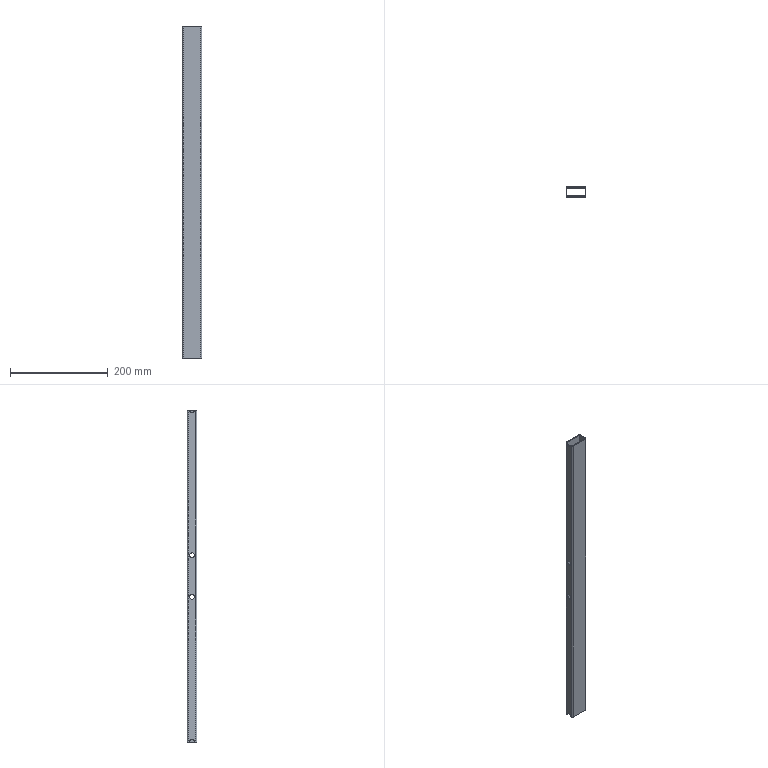Part | STEP file | 6150103 | 1 solid | 24 faces | box 40 x 20 x 680 mm | volume 112626 mm3 | cylinder 14 | plane 10 | commonest cylinder face diameters 10 x6 2 x4 5 x4
STEP:
#1=CARTESIAN_POINT('',(-18.5,-5.,340.));
#2=VERTEX_POINT('',#1);
#3=CARTESIAN_POINT('',(-18.5,-7.5,340.));
#4=VERTEX_POINT('',#3);
#5=CARTESIAN_POINT('',(-18.5,7.5,340.));
#6=DIRECTION('',(0.,-1.,0.));
#7=VECTOR('',#6,1000.);
#8=LINE('',#5,#7);
#9=EDGE_CURVE('',#2,#4,#8,.T.);
#10=ORIENTED_EDGE('',*,*,#9,.F.);
#11=CARTESIAN_POINT('',(-20.,-5.,340.));
#12=VERTEX_POINT('',#11);
#13=CARTESIAN_POINT('',(-10.,-5.,340.));
#14=DIRECTION('',(-1.,0.,0.));
#15=VECTOR('',#14,1000.);
#16=LINE('',#13,#15);
#17=EDGE_CURVE('',#2,#12,#16,.T.);
#18=ORIENTED_EDGE('',*,*,#17,.T.);
#19=CARTESIAN_POINT('',(-20.,-7.5,340.));
#20=VERTEX_POINT('',#19);
#21=CARTESIAN_POINT('',(-20.,7.5,340.));
#22=DIRECTION('',(0.,-1.,0.));
#23=VECTOR('',#22,1000.);
#24=LINE('',#21,#23);
#25=EDGE_CURVE('',#12,#20,#24,.T.);
#26=ORIENTED_EDGE('',*,*,#25,.T.);
#27=CARTESIAN_POINT('',(-17.5,-10.,340.));
#28=VERTEX_POINT('',#27);
#29=CARTESIAN_POINT('',(-17.5,-7.5,340.));
#30=DIRECTION('',(0.,0.,1.));
#31=DIRECTION('',(1.,0.,0.));
#32=AXIS2_PLACEMENT_3D('',#29,#30,#31);
#33=CIRCLE('',#32,2.5);
#34=EDGE_CURVE('',#20,#28,#33,.T.);
#35=ORIENTED_EDGE('',*,*,#34,.T.);
#36=CARTESIAN_POINT('',(17.5,-10.,340.));
#37=VERTEX_POINT('',#36);
#38=CARTESIAN_POINT('',(-17.5,-10.,340.));
#39=DIRECTION('',(1.,0.,0.));
#40=VECTOR('',#39,1000.);
#41=LINE('',#38,#40);
#42=EDGE_CURVE('',#28,#37,#41,.T.);
#43=ORIENTED_EDGE('',*,*,#42,.T.);
#44=CARTESIAN_POINT('',(20.,-7.5,340.));
#45=VERTEX_POINT('',#44);
#46=CARTESIAN_POINT('',(17.5,-7.5,340.));
#47=DIRECTION('',(0.,0.,1.));
#48=DIRECTION('',(1.,0.,0.));
#49=AXIS2_PLACEMENT_3D('',#46,#47,#48);
#50=CIRCLE('',#49,2.5);
#51=EDGE_CURVE('',#37,#45,#50,.T.);
#52=ORIENTED_EDGE('',*,*,#51,.T.);
#53=CARTESIAN_POINT('',(20.,7.5,340.));
#54=VERTEX_POINT('',#53);
#55=CARTESIAN_POINT('',(20.,7.5,340.));
#56=DIRECTION('',(0.,1.,0.));
#57=VECTOR('',#56,1000.);
#58=LINE('',#55,#57);
#59=EDGE_CURVE('',#45,#54,#58,.T.);
#60=ORIENTED_EDGE('',*,*,#59,.T.);
#61=CARTESIAN_POINT('',(17.5,10.,340.));
#62=VERTEX_POINT('',#61);
#63=CARTESIAN_POINT('',(17.5,7.5,340.));
#64=DIRECTION('',(0.,0.,1.));
#65=DIRECTION('',(-1.,0.,0.));
#66=AXIS2_PLACEMENT_3D('',#63,#64,#65);
#67=CIRCLE('',#66,2.5);
#68=EDGE_CURVE('',#54,#62,#67,.T.);
#69=ORIENTED_EDGE('',*,*,#68,.T.);
#70=CARTESIAN_POINT('',(-17.5,10.,340.));
#71=VERTEX_POINT('',#70);
#72=CARTESIAN_POINT('',(-17.5,10.,340.));
#73=DIRECTION('',(-1.,0.,0.));
#74=VECTOR('',#73,1000.);
#75=LINE('',#72,#74);
#76=EDGE_CURVE('',#62,#71,#75,.T.);
#77=ORIENTED_EDGE('',*,*,#76,.T.);
#78=CARTESIAN_POINT('',(-20.,7.5,340.));
#79=VERTEX_POINT('',#78);
#80=CARTESIAN_POINT('',(-17.5,7.5,340.));
#81=DIRECTION('',(0.,0.,1.));
#82=DIRECTION('',(1.,0.,0.));
#83=AXIS2_PLACEMENT_3D('',#80,#81,#82);
#84=CIRCLE('',#83,2.5);
#85=EDGE_CURVE('',#71,#79,#84,.T.);
#86=ORIENTED_EDGE('',*,*,#85,.T.);
#87=CARTESIAN_POINT('',(-20.,5.,340.));
#88=VERTEX_POINT('',#87);
#89=CARTESIAN_POINT('',(-20.,7.5,340.));
#90=DIRECTION('',(0.,-1.,0.));
#91=VECTOR('',#90,1000.);
#92=LINE('',#89,#91);
#93=EDGE_CURVE('',#79,#88,#92,.T.);
#94=ORIENTED_EDGE('',*,*,#93,.T.);
#95=CARTESIAN_POINT('',(-18.5,5.,340.));
#96=VERTEX_POINT('',#95);
#97=CARTESIAN_POINT('',(-10.,5.,340.));
#98=DIRECTION('',(1.,0.,0.));
#99=VECTOR('',#98,1000.);
#100=LINE('',#97,#99);
#101=EDGE_CURVE('',#88,#96,#100,.T.);
#102=ORIENTED_EDGE('',*,*,#101,.T.);
#103=CARTESIAN_POINT('',(-18.5,7.5,340.));
#104=VERTEX_POINT('',#103);
#105=CARTESIAN_POINT('',(-18.5,7.5,340.));
#106=DIRECTION('',(0.,-1.,0.));
#107=VECTOR('',#106,1000.);
#108=LINE('',#105,#107);
#109=EDGE_CURVE('',#104,#96,#108,.T.);
#110=ORIENTED_EDGE('',*,*,#109,.F.);
#111=CARTESIAN_POINT('',(-17.5,8.5,340.));
#112=VERTEX_POINT('',#111);
#113=CARTESIAN_POINT('',(-17.5,7.5,340.));
#114=DIRECTION('',(0.,0.,1.));
#115=DIRECTION('',(1.,0.,0.));
#116=AXIS2_PLACEMENT_3D('',#113,#114,#115);
#117=CIRCLE('',#116,1.);
#118=EDGE_CURVE('',#112,#104,#117,.T.);
#119=ORIENTED_EDGE('',*,*,#118,.F.);
#120=CARTESIAN_POINT('',(17.5,8.5,340.));
#121=VERTEX_POINT('',#120);
#122=CARTESIAN_POINT('',(-17.5,8.5,340.));
#123=DIRECTION('',(-1.,0.,0.));
#124=VECTOR('',#123,1000.);
#125=LINE('',#122,#124);
#126=EDGE_CURVE('',#121,#112,#125,.T.);
#127=ORIENTED_EDGE('',*,*,#126,.F.);
#128=CARTESIAN_POINT('',(18.5,7.5,340.));
#129=VERTEX_POINT('',#128);
#130=CARTESIAN_POINT('',(17.5,7.5,340.));
#131=DIRECTION('',(0.,0.,1.));
#132=DIRECTION('',(-1.,0.,0.));
#133=AXIS2_PLACEMENT_3D('',#130,#131,#132);
#134=CIRCLE('',#133,1.);
#135=EDGE_CURVE('',#129,#121,#134,.T.);
#136=ORIENTED_EDGE('',*,*,#135,.F.);
#137=CARTESIAN_POINT('',(18.5,-7.5,340.));
#138=VERTEX_POINT('',#137);
#139=CARTESIAN_POINT('',(18.5,7.5,340.));
#140=DIRECTION('',(0.,1.,0.));
#141=VECTOR('',#140,1000.);
#142=LINE('',#139,#141);
#143=EDGE_CURVE('',#138,#129,#142,.T.);
#144=ORIENTED_EDGE('',*,*,#143,.F.);
#145=CARTESIAN_POINT('',(17.5,-8.5,340.));
#146=VERTEX_POINT('',#145);
#147=CARTESIAN_POINT('',(17.5,-7.5,340.));
#148=DIRECTION('',(0.,0.,1.));
#149=DIRECTION('',(1.,0.,0.));
#150=AXIS2_PLACEMENT_3D('',#147,#148,#149);
#151=CIRCLE('',#150,1.);
#152=EDGE_CURVE('',#146,#138,#151,.T.);
#153=ORIENTED_EDGE('',*,*,#152,.F.);
#154=CARTESIAN_POINT('',(-17.5,-8.5,340.));
#155=VERTEX_POINT('',#154);
#156=CARTESIAN_POINT('',(-17.5,-8.5,340.));
#157=DIRECTION('',(1.,0.,0.));
#158=VECTOR('',#157,1000.);
#159=LINE('',#156,#158);
#160=EDGE_CURVE('',#155,#146,#159,.T.);
#161=ORIENTED_EDGE('',*,*,#160,.F.);
#162=CARTESIAN_POINT('',(-17.5,-7.5,340.));
#163=DIRECTION('',(0.,0.,1.));
#164=DIRECTION('',(1.,0.,0.));
#165=AXIS2_PLACEMENT_3D('',#162,#163,#164);
#166=CIRCLE('',#165,1.);
#167=EDGE_CURVE('',#4,#155,#166,.T.);
#168=ORIENTED_EDGE('',*,*,#167,.F.);
#169=EDGE_LOOP('',(#10,#18,#26,#35,#43,#52,#60,#69,#77,#86,#94,#102,#110,#119,#127,#136,#144,#153,#161,#168));
#170=FACE_OUTER_BOUND('',#169,.T.);
#171=CARTESIAN_POINT('',(17.5,7.5,340.));
#172=DIRECTION('',(0.,0.,-1.));
#173=DIRECTION('',(-1.,0.,0.));
#174=AXIS2_PLACEMENT_3D('',#171,#172,#173);
#175=PLANE('',#174);
#176=ADVANCED_FACE('',(#170),#175,.F.);
#177=CARTESIAN_POINT('',(-18.5,-5.,-340.));
#178=VERTEX_POINT('',#177);
#179=CARTESIAN_POINT('',(-20.,-5.,-340.));
#180=VERTEX_POINT('',#179);
#181=CARTESIAN_POINT('',(-10.,-5.,-340.));
#182=DIRECTION('',(-1.,0.,0.));
#183=VECTOR('',#182,1000.);
#184=LINE('',#181,#183);
#185=EDGE_CURVE('',#178,#180,#184,.T.);
#186=ORIENTED_EDGE('',*,*,#185,.F.);
#187=CARTESIAN_POINT('',(-18.5,-7.5,-340.));
#188=VERTEX_POINT('',#187);
#189=CARTESIAN_POINT('',(-18.5,7.5,-340.));
#190=DIRECTION('',(0.,-1.,0.));
#191=VECTOR('',#190,1000.);
#192=LINE('',#189,#191);
#193=EDGE_CURVE('',#178,#188,#192,.T.);
#194=ORIENTED_EDGE('',*,*,#193,.T.);
#195=CARTESIAN_POINT('',(-17.5,-8.5,-340.));
#196=VERTEX_POINT('',#195);
#197=CARTESIAN_POINT('',(-17.5,-7.5,-340.));
#198=DIRECTION('',(0.,0.,1.));
#199=DIRECTION('',(1.,0.,0.));
#200=AXIS2_PLACEMENT_3D('',#197,#198,#199);
#201=CIRCLE('',#200,1.);
#202=EDGE_CURVE('',#188,#196,#201,.T.);
#203=ORIENTED_EDGE('',*,*,#202,.T.);
#204=CARTESIAN_POINT('',(17.5,-8.5,-340.));
#205=VERTEX_POINT('',#204);
#206=CARTESIAN_POINT('',(-17.5,-8.5,-340.));
#207=DIRECTION('',(1.,0.,0.));
#208=VECTOR('',#207,1000.);
#209=LINE('',#206,#208);
#210=EDGE_CURVE('',#196,#205,#209,.T.);
#211=ORIENTED_EDGE('',*,*,#210,.T.);
#212=CARTESIAN_POINT('',(18.5,-7.5,-340.));
#213=VERTEX_POINT('',#212);
#214=CARTESIAN_POINT('',(17.5,-7.5,-340.));
#215=DIRECTION('',(0.,0.,1.));
#216=DIRECTION('',(1.,0.,0.));
#217=AXIS2_PLACEMENT_3D('',#214,#215,#216);
#218=CIRCLE('',#217,1.);
#219=EDGE_CURVE('',#205,#213,#218,.T.);
#220=ORIENTED_EDGE('',*,*,#219,.T.);
#221=CARTESIAN_POINT('',(18.5,7.5,-340.));
#222=VERTEX_POINT('',#221);
#223=CARTESIAN_POINT('',(18.5,7.5,-340.));
#224=DIRECTION('',(0.,1.,0.));
#225=VECTOR('',#224,1000.);
#226=LINE('',#223,#225);
#227=EDGE_CURVE('',#213,#222,#226,.T.);
#228=ORIENTED_EDGE('',*,*,#227,.T.);
#229=CARTESIAN_POINT('',(17.5,8.5,-340.));
#230=VERTEX_POINT('',#229);
#231=CARTESIAN_POINT('',(17.5,7.5,-340.));
#232=DIRECTION('',(0.,0.,1.));
#233=DIRECTION('',(-1.,0.,0.));
#234=AXIS2_PLACEMENT_3D('',#231,#232,#233);
#235=CIRCLE('',#234,1.);
#236=EDGE_CURVE('',#222,#230,#235,.T.);
#237=ORIENTED_EDGE('',*,*,#236,.T.);
#238=CARTESIAN_POINT('',(-17.5,8.5,-340.));
#239=VERTEX_POINT('',#238);
#240=CARTESIAN_POINT('',(-17.5,8.5,-340.));
#241=DIRECTION('',(-1.,0.,0.));
#242=VECTOR('',#241,1000.);
#243=LINE('',#240,#242);
#244=EDGE_CURVE('',#230,#239,#243,.T.);
#245=ORIENTED_EDGE('',*,*,#244,.T.);
#246=CARTESIAN_POINT('',(-18.5,7.5,-340.));
#247=VERTEX_POINT('',#246);
#248=CARTESIAN_POINT('',(-17.5,7.5,-340.));
#249=DIRECTION('',(0.,0.,1.));
#250=DIRECTION('',(1.,0.,0.));
#251=AXIS2_PLACEMENT_3D('',#248,#249,#250);
#252=CIRCLE('',#251,1.);
#253=EDGE_CURVE('',#239,#247,#252,.T.);
#254=ORIENTED_EDGE('',*,*,#253,.T.);
#255=CARTESIAN_POINT('',(-18.5,5.,-340.));
#256=VERTEX_POINT('',#255);
#257=CARTESIAN_POINT('',(-18.5,7.5,-340.));
#258=DIRECTION('',(0.,-1.,0.));
#259=VECTOR('',#258,1000.);
#260=LINE('',#257,#259);
#261=EDGE_CURVE('',#247,#256,#260,.T.);
#262=ORIENTED_EDGE('',*,*,#261,.T.);
#263=CARTESIAN_POINT('',(-20.,5.,-340.));
#264=VERTEX_POINT('',#263);
#265=CARTESIAN_POINT('',(-10.,5.,-340.));
#266=DIRECTION('',(1.,0.,0.));
#267=VECTOR('',#266,1000.);
#268=LINE('',#265,#267);
#269=EDGE_CURVE('',#264,#256,#268,.T.);
#270=ORIENTED_EDGE('',*,*,#269,.F.);
#271=CARTESIAN_POINT('',(-20.,7.5,-340.));
#272=VERTEX_POINT('',#271);
#273=CARTESIAN_POINT('',(-20.,7.5,-340.));
#274=DIRECTION('',(0.,-1.,0.));
#275=VECTOR('',#274,1000.);
#276=LINE('',#273,#275);
#277=EDGE_CURVE('',#272,#264,#276,.T.);
#278=ORIENTED_EDGE('',*,*,#277,.F.);
#279=CARTESIAN_POINT('',(-17.5,10.,-340.));
#280=VERTEX_POINT('',#279);
#281=CARTESIAN_POINT('',(-17.5,7.5,-340.));
#282=DIRECTION('',(0.,0.,1.));
#283=DIRECTION('',(1.,0.,0.));
#284=AXIS2_PLACEMENT_3D('',#281,#282,#283);
#285=CIRCLE('',#284,2.5);
#286=EDGE_CURVE('',#280,#272,#285,.T.);
#287=ORIENTED_EDGE('',*,*,#286,.F.);
#288=CARTESIAN_POINT('',(17.5,10.,-340.));
#289=VERTEX_POINT('',#288);
#290=CARTESIAN_POINT('',(-17.5,10.,-340.));
#291=DIRECTION('',(-1.,0.,0.));
#292=VECTOR('',#291,1000.);
#293=LINE('',#290,#292);
#294=EDGE_CURVE('',#289,#280,#293,.T.);
#295=ORIENTED_EDGE('',*,*,#294,.F.);
#296=CARTESIAN_POINT('',(20.,7.5,-340.));
#297=VERTEX_POINT('',#296);
#298=CARTESIAN_POINT('',(17.5,7.5,-340.));
#299=DIRECTION('',(0.,0.,1.));
#300=DIRECTION('',(-1.,0.,0.));
#301=AXIS2_PLACEMENT_3D('',#298,#299,#300);
#302=CIRCLE('',#301,2.5);
#303=EDGE_CURVE('',#297,#289,#302,.T.);
#304=ORIENTED_EDGE('',*,*,#303,.F.);
#305=CARTESIAN_POINT('',(20.,-7.5,-340.));
#306=VERTEX_POINT('',#305);
#307=CARTESIAN_POINT('',(20.,7.5,-340.));
#308=DIRECTION('',(0.,1.,0.));
#309=VECTOR('',#308,1000.);
#310=LINE('',#307,#309);
#311=EDGE_CURVE('',#306,#297,#310,.T.);
#312=ORIENTED_EDGE('',*,*,#311,.F.);
#313=CARTESIAN_POINT('',(17.5,-10.,-340.));
#314=VERTEX_POINT('',#313);
#315=CARTESIAN_POINT('',(17.5,-7.5,-340.));
#316=DIRECTION('',(0.,0.,1.));
#317=DIRECTION('',(1.,0.,0.));
#318=AXIS2_PLACEMENT_3D('',#315,#316,#317);
#319=CIRCLE('',#318,2.5);
#320=EDGE_CURVE('',#314,#306,#319,.T.);
#321=ORIENTED_EDGE('',*,*,#320,.F.);
#322=CARTESIAN_POINT('',(-17.5,-10.,-340.));
#323=VERTEX_POINT('',#322);
#324=CARTESIAN_POINT('',(-17.5,-10.,-340.));
#325=DIRECTION('',(1.,0.,0.));
#326=VECTOR('',#325,1000.);
#327=LINE('',#324,#326);
#328=EDGE_CURVE('',#323,#314,#327,.T.);
#329=ORIENTED_EDGE('',*,*,#328,.F.);
#330=CARTESIAN_POINT('',(-20.,-7.5,-340.));
#331=VERTEX_POINT('',#330);
#332=CARTESIAN_POINT('',(-17.5,-7.5,-340.));
#333=DIRECTION('',(0.,0.,1.));
#334=DIRECTION('',(1.,0.,0.));
#335=AXIS2_PLACEMENT_3D('',#332,#333,#334);
#336=CIRCLE('',#335,2.5);
#337=EDGE_CURVE('',#331,#323,#336,.T.);
#338=ORIENTED_EDGE('',*,*,#337,.F.);
#339=CARTESIAN_POINT('',(-20.,7.5,-340.));
#340=DIRECTION('',(0.,-1.,0.));
#341=VECTOR('',#340,1000.);
#342=LINE('',#339,#341);
#343=EDGE_CURVE('',#180,#331,#342,.T.);
#344=ORIENTED_EDGE('',*,*,#343,.F.);
#345=EDGE_LOOP('',(#186,#194,#203,#211,#220,#228,#237,#245,#254,#262,#270,#278,#287,#295,#304,#312,#321,#329,#338,#344));
#346=FACE_OUTER_BOUND('',#345,.T.);
#347=CARTESIAN_POINT('',(17.5,7.5,-340.));
#348=DIRECTION('',(0.,0.,-1.));
#349=DIRECTION('',(-1.,0.,0.));
#350=AXIS2_PLACEMENT_3D('',#347,#348,#349);
#351=PLANE('',#350);
#352=ADVANCED_FACE('',(#346),#351,.T.);
#353=ORIENTED_EDGE('',*,*,#303,.T.);
#354=CARTESIAN_POINT('',(17.5,10.,340.));
#355=DIRECTION('',(0.,0.,-1.));
#356=VECTOR('',#355,1000.);
#357=LINE('',#354,#356);
#358=EDGE_CURVE('',#62,#289,#357,.T.);
#359=ORIENTED_EDGE('',*,*,#358,.F.);
#360=ORIENTED_EDGE('',*,*,#68,.F.);
#361=CARTESIAN_POINT('',(20.,7.5,340.));
#362=DIRECTION('',(0.,0.,-1.));
#363=VECTOR('',#362,1000.);
#364=LINE('',#361,#363);
#365=EDGE_CURVE('',#54,#297,#364,.T.);
#366=ORIENTED_EDGE('',*,*,#365,.T.);
#367=EDGE_LOOP('',(#353,#359,#360,#366));
#368=FACE_OUTER_BOUND('',#367,.T.);
#369=CARTESIAN_POINT('',(17.5,7.5,340.));
#370=DIRECTION('',(0.,0.,-1.));
#371=DIRECTION('',(-1.,0.,0.));
#372=AXIS2_PLACEMENT_3D('',#369,#370,#371);
#373=CYLINDRICAL_SURFACE('',#372,2.5);
#374=ADVANCED_FACE('',(#368),#373,.T.);
#375=ORIENTED_EDGE('',*,*,#294,.T.);
#376=CARTESIAN_POINT('',(-17.5,10.,340.));
#377=DIRECTION('',(0.,0.,-1.));
#378=VECTOR('',#377,1000.);
#379=LINE('',#376,#378);
#380=EDGE_CURVE('',#71,#280,#379,.T.);
#381=ORIENTED_EDGE('',*,*,#380,.F.);
#382=ORIENTED_EDGE('',*,*,#76,.F.);
#383=ORIENTED_EDGE('',*,*,#358,.T.);
#384=EDGE_LOOP('',(#375,#381,#382,#383));
#385=FACE_OUTER_BOUND('',#384,.T.);
#386=CARTESIAN_POINT('',(-17.5,10.,340.));
#387=DIRECTION('',(0.,-1.,0.));
#388=DIRECTION('',(0.,0.,-1.));
#389=AXIS2_PLACEMENT_3D('',#386,#387,#388);
#390=PLANE('',#389);
#391=ADVANCED_FACE('',(#385),#390,.F.);
#392=ORIENTED_EDGE('',*,*,#286,.T.);
#393=CARTESIAN_POINT('',(-20.,7.5,340.));
#394=DIRECTION('',(0.,0.,-1.));
#395=VECTOR('',#394,1000.);
#396=LINE('',#393,#395);
#397=EDGE_CURVE('',#79,#272,#396,.T.);
#398=ORIENTED_EDGE('',*,*,#397,.F.);
#399=ORIENTED_EDGE('',*,*,#85,.F.);
#400=ORIENTED_EDGE('',*,*,#380,.T.);
#401=EDGE_LOOP('',(#392,#398,#399,#400));
#402=FACE_OUTER_BOUND('',#401,.T.);
#403=CARTESIAN_POINT('',(-17.5,7.5,340.));
#404=DIRECTION('',(0.,0.,-1.));
#405=DIRECTION('',(-1.,0.,0.));
#406=AXIS2_PLACEMENT_3D('',#403,#404,#405);
#407=CYLINDRICAL_SURFACE('',#406,2.5);
#408=ADVANCED_FACE('',(#402),#407,.T.);
#409=CARTESIAN_POINT('',(-20.,-5.,42.5));
#410=VERTEX_POINT('',#409);
#411=CARTESIAN_POINT('',(-20.,0.,42.5));
#412=DIRECTION('',(-1.,0.,0.));
#413=DIRECTION('',(0.,-1.,0.));
#414=AXIS2_PLACEMENT_3D('',#411,#412,#413);
#415=CIRCLE('',#414,5.);
#416=EDGE_CURVE('',#410,#410,#415,.T.);
#417=ORIENTED_EDGE('',*,*,#416,.F.);
#418=EDGE_LOOP('',(#417));
#419=FACE_BOUND('',#418,.T.);
#420=CARTESIAN_POINT('',(-20.,-5.,-42.5));
#421=VERTEX_POINT('',#420);
#422=CARTESIAN_POINT('',(-20.,0.,-42.5));
#423=DIRECTION('',(-1.,0.,0.));
#424=DIRECTION('',(0.,-1.,0.));
#425=AXIS2_PLACEMENT_3D('',#422,#423,#424);
#426=CIRCLE('',#425,5.);
#427=EDGE_CURVE('',#421,#421,#426,.T.);
#428=ORIENTED_EDGE('',*,*,#427,.F.);
#429=EDGE_LOOP('',(#428));
#430=FACE_BOUND('',#429,.T.);
#431=ORIENTED_EDGE('',*,*,#277,.T.);
#432=CARTESIAN_POINT('',(-20.,0.,-340.));
#433=DIRECTION('',(-1.,0.,0.));
#434=DIRECTION('',(0.,-1.,0.));
#435=AXIS2_PLACEMENT_3D('',#432,#433,#434);
#436=CIRCLE('',#435,5.);
#437=EDGE_CURVE('',#180,#264,#436,.T.);
#438=ORIENTED_EDGE('',*,*,#437,.F.);
#439=ORIENTED_EDGE('',*,*,#343,.T.);
#440=CARTESIAN_POINT('',(-20.,-7.5,340.));
#441=DIRECTION('',(0.,0.,-1.));
#442=VECTOR('',#441,1000.);
#443=LINE('',#440,#442);
#444=EDGE_CURVE('',#20,#331,#443,.T.);
#445=ORIENTED_EDGE('',*,*,#444,.F.);
#446=ORIENTED_EDGE('',*,*,#25,.F.);
#447=CARTESIAN_POINT('',(-20.,0.,340.));
#448=DIRECTION('',(-1.,0.,0.));
#449=DIRECTION('',(0.,-1.,0.));
#450=AXIS2_PLACEMENT_3D('',#447,#448,#449);
#451=CIRCLE('',#450,5.);
#452=EDGE_CURVE('',#88,#12,#451,.T.);
#453=ORIENTED_EDGE('',*,*,#452,.F.);
#454=ORIENTED_EDGE('',*,*,#93,.F.);
#455=ORIENTED_EDGE('',*,*,#397,.T.);
#456=EDGE_LOOP('',(#431,#438,#439,#445,#446,#453,#454,#455));
#457=FACE_OUTER_BOUND('',#456,.T.);
#458=CARTESIAN_POINT('',(-20.,7.5,340.));
#459=DIRECTION('',(1.,0.,0.));
#460=DIRECTION('',(0.,1.,0.));
#461=AXIS2_PLACEMENT_3D('',#458,#459,#460);
#462=PLANE('',#461);
#463=ADVANCED_FACE('',(#419,#430,#457),#462,.F.);
#464=ORIENTED_EDGE('',*,*,#337,.T.);
#465=CARTESIAN_POINT('',(-17.5,-10.,340.));
#466=DIRECTION('',(0.,0.,-1.));
#467=VECTOR('',#466,1000.);
#468=LINE('',#465,#467);
#469=EDGE_CURVE('',#28,#323,#468,.T.);
#470=ORIENTED_EDGE('',*,*,#469,.F.);
#471=ORIENTED_EDGE('',*,*,#34,.F.);
#472=ORIENTED_EDGE('',*,*,#444,.T.);
#473=EDGE_LOOP('',(#464,#470,#471,#472));
#474=FACE_OUTER_BOUND('',#473,.T.);
#475=CARTESIAN_POINT('',(-17.5,-7.5,340.));
#476=DIRECTION('',(0.,0.,-1.));
#477=DIRECTION('',(-1.,0.,0.));
#478=AXIS2_PLACEMENT_3D('',#475,#476,#477);
#479=CYLINDRICAL_SURFACE('',#478,2.5);
#480=ADVANCED_FACE('',(#474),#479,.T.);
#481=ORIENTED_EDGE('',*,*,#328,.T.);
#482=CARTESIAN_POINT('',(17.5,-10.,340.));
#483=DIRECTION('',(0.,0.,-1.));
#484=VECTOR('',#483,1000.);
#485=LINE('',#482,#484);
#486=EDGE_CURVE('',#37,#314,#485,.T.);
#487=ORIENTED_EDGE('',*,*,#486,.F.);
#488=ORIENTED_EDGE('',*,*,#42,.F.);
#489=ORIENTED_EDGE('',*,*,#469,.T.);
#490=EDGE_LOOP('',(#481,#487,#488,#489));
#491=FACE_OUTER_BOUND('',#490,.T.);
#492=CARTESIAN_POINT('',(-17.5,-10.,340.));
#493=DIRECTION('',(0.,1.,0.));
#494=DIRECTION('',(0.,0.,1.));
#495=AXIS2_PLACEMENT_3D('',#492,#493,#494);
#496=PLANE('',#495);
#497=ADVANCED_FACE('',(#491),#496,.F.);
#498=ORIENTED_EDGE('',*,*,#320,.T.);
#499=CARTESIAN_POINT('',(20.,-7.5,340.));
#500=DIRECTION('',(0.,0.,-1.));
#501=VECTOR('',#500,1000.);
#502=LINE('',#499,#501);
#503=EDGE_CURVE('',#45,#306,#502,.T.);
#504=ORIENTED_EDGE('',*,*,#503,.F.);
#505=ORIENTED_EDGE('',*,*,#51,.F.);
#506=ORIENTED_EDGE('',*,*,#486,.T.);
#507=EDGE_LOOP('',(#498,#504,#505,#506));
#508=FACE_OUTER_BOUND('',#507,.T.);
#509=CARTESIAN_POINT('',(17.5,-7.5,340.));
#510=DIRECTION('',(0.,0.,-1.));
#511=DIRECTION('',(-1.,0.,0.));
#512=AXIS2_PLACEMENT_3D('',#509,#510,#511);
#513=CYLINDRICAL_SURFACE('',#512,2.5);
#514=ADVANCED_FACE('',(#508),#513,.T.);
#515=CARTESIAN_POINT('',(20.,-5.,42.5));
#516=VERTEX_POINT('',#515);
#517=CARTESIAN_POINT('',(20.,0.,42.5));
#518=DIRECTION('',(-1.,0.,0.));
#519=DIRECTION('',(0.,-1.,0.));
#520=AXIS2_PLACEMENT_3D('',#517,#518,#519);
#521=CIRCLE('',#520,5.);
#522=EDGE_CURVE('',#516,#516,#521,.T.);
#523=ORIENTED_EDGE('',*,*,#522,.T.);
#524=EDGE_LOOP('',(#523));
#525=FACE_BOUND('',#524,.T.);
#526=CARTESIAN_POINT('',(20.,-5.,-42.5));
#527=VERTEX_POINT('',#526);
#528=CARTESIAN_POINT('',(20.,0.,-42.5));
#529=DIRECTION('',(-1.,0.,0.));
#530=DIRECTION('',(0.,-1.,0.));
#531=AXIS2_PLACEMENT_3D('',#528,#529,#530);
#532=CIRCLE('',#531,5.);
#533=EDGE_CURVE('',#527,#527,#532,.T.);
#534=ORIENTED_EDGE('',*,*,#533,.T.);
#535=EDGE_LOOP('',(#534));
#536=FACE_BOUND('',#535,.T.);
#537=ORIENTED_EDGE('',*,*,#311,.T.);
#538=ORIENTED_EDGE('',*,*,#365,.F.);
#539=ORIENTED_EDGE('',*,*,#59,.F.);
#540=ORIENTED_EDGE('',*,*,#503,.T.);
#541=EDGE_LOOP('',(#537,#538,#539,#540));
#542=FACE_OUTER_BOUND('',#541,.T.);
#543=CARTESIAN_POINT('',(20.,7.5,340.));
#544=DIRECTION('',(-1.,0.,0.));
#545=DIRECTION('',(0.,-1.,0.));
#546=AXIS2_PLACEMENT_3D('',#543,#544,#545);
#547=PLANE('',#546);
#548=ADVANCED_FACE('',(#525,#536,#542),#547,.F.);
#549=ORIENTED_EDGE('',*,*,#253,.F.);
#550=CARTESIAN_POINT('',(-17.5,8.5,340.));
#551=DIRECTION('',(0.,0.,-1.));
#552=VECTOR('',#551,1000.);
#553=LINE('',#550,#552);
#554=EDGE_CURVE('',#112,#239,#553,.T.);
#555=ORIENTED_EDGE('',*,*,#554,.F.);
#556=ORIENTED_EDGE('',*,*,#118,.T.);
#557=CARTESIAN_POINT('',(-18.5,7.5,340.));
#558=DIRECTION('',(0.,0.,-1.));
#559=VECTOR('',#558,1000.);
#560=LINE('',#557,#559);
#561=EDGE_CURVE('',#104,#247,#560,.T.);
#562=ORIENTED_EDGE('',*,*,#561,.T.);
#563=EDGE_LOOP('',(#549,#555,#556,#562));
#564=FACE_OUTER_BOUND('',#563,.T.);
#565=CARTESIAN_POINT('',(-17.5,7.5,340.));
#566=DIRECTION('',(0.,0.,-1.));
#567=DIRECTION('',(-1.,0.,0.));
#568=AXIS2_PLACEMENT_3D('',#565,#566,#567);
#569=CYLINDRICAL_SURFACE('',#568,1.);
#570=ADVANCED_FACE('',(#564),#569,.F.);
#571=CARTESIAN_POINT('',(-18.5,0.,37.5));
#572=VERTEX_POINT('',#571);
#573=CARTESIAN_POINT('',(-18.5,0.,42.5));
#574=DIRECTION('',(1.,0.,0.));
#575=DIRECTION('',(0.,0.,-1.));
#576=AXIS2_PLACEMENT_3D('',#573,#574,#575);
#577=CIRCLE('',#576,5.);
#578=EDGE_CURVE('',#572,#572,#577,.T.);
#579=ORIENTED_EDGE('',*,*,#578,.F.);
#580=EDGE_LOOP('',(#579));
#581=FACE_BOUND('',#580,.T.);
#582=CARTESIAN_POINT('',(-18.5,0.,-47.5));
#583=VERTEX_POINT('',#582);
#584=CARTESIAN_POINT('',(-18.5,0.,-42.5));
#585=DIRECTION('',(1.,0.,0.));
#586=DIRECTION('',(0.,0.,-1.));
#587=AXIS2_PLACEMENT_3D('',#584,#585,#586);
#588=CIRCLE('',#587,5.);
#589=EDGE_CURVE('',#583,#583,#588,.T.);
#590=ORIENTED_EDGE('',*,*,#589,.F.);
#591=EDGE_LOOP('',(#590));
#592=FACE_BOUND('',#591,.T.);
#593=CARTESIAN_POINT('',(-18.5,0.,-340.));
#594=DIRECTION('',(1.,0.,0.));
#595=DIRECTION('',(0.,0.,-1.));
#596=AXIS2_PLACEMENT_3D('',#593,#594,#595);
#597=CIRCLE('',#596,5.);
#598=EDGE_CURVE('',#256,#178,#597,.T.);
#599=ORIENTED_EDGE('',*,*,#598,.F.);
#600=ORIENTED_EDGE('',*,*,#261,.F.);
#601=ORIENTED_EDGE('',*,*,#561,.F.);
#602=ORIENTED_EDGE('',*,*,#109,.T.);
#603=CARTESIAN_POINT('',(-18.5,0.,340.));
#604=DIRECTION('',(1.,0.,0.));
#605=DIRECTION('',(0.,0.,-1.));
#606=AXIS2_PLACEMENT_3D('',#603,#604,#605);
#607=CIRCLE('',#606,5.);
#608=EDGE_CURVE('',#2,#96,#607,.T.);
#609=ORIENTED_EDGE('',*,*,#608,.F.);
#610=ORIENTED_EDGE('',*,*,#9,.T.);
#611=CARTESIAN_POINT('',(-18.5,-7.5,340.));
#612=DIRECTION('',(0.,0.,-1.));
#613=VECTOR('',#612,1000.);
#614=LINE('',#611,#613);
#615=EDGE_CURVE('',#4,#188,#614,.T.);
#616=ORIENTED_EDGE('',*,*,#615,.T.);
#617=ORIENTED_EDGE('',*,*,#193,.F.);
#618=EDGE_LOOP('',(#599,#600,#601,#602,#609,#610,#616,#617));
#619=FACE_OUTER_BOUND('',#618,.T.);
#620=CARTESIAN_POINT('',(-18.5,7.5,340.));
#621=DIRECTION('',(1.,0.,0.));
#622=DIRECTION('',(0.,0.,-1.));
#623=AXIS2_PLACEMENT_3D('',#620,#621,#622);
#624=PLANE('',#623);
#625=ADVANCED_FACE('',(#581,#592,#619),#624,.T.);
#626=ORIENTED_EDGE('',*,*,#202,.F.);
#627=ORIENTED_EDGE('',*,*,#615,.F.);
#628=ORIENTED_EDGE('',*,*,#167,.T.);
#629=CARTESIAN_POINT('',(-17.5,-8.5,340.));
#630=DIRECTION('',(0.,0.,-1.));
#631=VECTOR('',#630,1000.);
#632=LINE('',#629,#631);
#633=EDGE_CURVE('',#155,#196,#632,.T.);
#634=ORIENTED_EDGE('',*,*,#633,.T.);
#635=EDGE_LOOP('',(#626,#627,#628,#634));
#636=FACE_OUTER_BOUND('',#635,.T.);
#637=CARTESIAN_POINT('',(-17.5,-7.5,340.));
#638=DIRECTION('',(0.,0.,-1.));
#639=DIRECTION('',(-1.,0.,0.));
#640=AXIS2_PLACEMENT_3D('',#637,#638,#639);
#641=CYLINDRICAL_SURFACE('',#640,1.);
#642=ADVANCED_FACE('',(#636),#641,.F.);
#643=ORIENTED_EDGE('',*,*,#210,.F.);
#644=ORIENTED_EDGE('',*,*,#633,.F.);
#645=ORIENTED_EDGE('',*,*,#160,.T.);
#646=CARTESIAN_POINT('',(17.5,-8.5,340.));
#647=DIRECTION('',(0.,0.,-1.));
#648=VECTOR('',#647,1000.);
#649=LINE('',#646,#648);
#650=EDGE_CURVE('',#146,#205,#649,.T.);
#651=ORIENTED_EDGE('',*,*,#650,.T.);
#652=EDGE_LOOP('',(#643,#644,#645,#651));
#653=FACE_OUTER_BOUND('',#652,.T.);
#654=CARTESIAN_POINT('',(-17.5,-8.5,340.));
#655=DIRECTION('',(0.,1.,0.));
#656=DIRECTION('',(-1.,0.,0.));
#657=AXIS2_PLACEMENT_3D('',#654,#655,#656);
#658=PLANE('',#657);
#659=ADVANCED_FACE('',(#653),#658,.T.);
#660=ORIENTED_EDGE('',*,*,#219,.F.);
#661=ORIENTED_EDGE('',*,*,#650,.F.);
#662=ORIENTED_EDGE('',*,*,#152,.T.);
#663=CARTESIAN_POINT('',(18.5,-7.5,340.));
#664=DIRECTION('',(0.,0.,-1.));
#665=VECTOR('',#664,1000.);
#666=LINE('',#663,#665);
#667=EDGE_CURVE('',#138,#213,#666,.T.);
#668=ORIENTED_EDGE('',*,*,#667,.T.);
#669=EDGE_LOOP('',(#660,#661,#662,#668));
#670=FACE_OUTER_BOUND('',#669,.T.);
#671=CARTESIAN_POINT('',(17.5,-7.5,340.));
#672=DIRECTION('',(0.,0.,-1.));
#673=DIRECTION('',(-1.,0.,0.));
#674=AXIS2_PLACEMENT_3D('',#671,#672,#673);
#675=CYLINDRICAL_SURFACE('',#674,1.);
#676=ADVANCED_FACE('',(#670),#675,.F.);
#677=CARTESIAN_POINT('',(18.5,-5.,42.5));
#678=VERTEX_POINT('',#677);
#679=CARTESIAN_POINT('',(18.5,0.,42.5));
#680=DIRECTION('',(-1.,0.,0.));
#681=DIRECTION('',(0.,-1.,0.));
#682=AXIS2_PLACEMENT_3D('',#679,#680,#681);
#683=CIRCLE('',#682,5.);
#684=EDGE_CURVE('',#678,#678,#683,.T.);
#685=ORIENTED_EDGE('',*,*,#684,.F.);
#686=EDGE_LOOP('',(#685));
#687=FACE_BOUND('',#686,.T.);
#688=CARTESIAN_POINT('',(18.5,-5.,-42.5));
#689=VERTEX_POINT('',#688);
#690=CARTESIAN_POINT('',(18.5,0.,-42.5));
#691=DIRECTION('',(-1.,0.,0.));
#692=DIRECTION('',(0.,-1.,0.));
#693=AXIS2_PLACEMENT_3D('',#690,#691,#692);
#694=CIRCLE('',#693,5.);
#695=EDGE_CURVE('',#689,#689,#694,.T.);
#696=ORIENTED_EDGE('',*,*,#695,.F.);
#697=EDGE_LOOP('',(#696));
#698=FACE_BOUND('',#697,.T.);
#699=ORIENTED_EDGE('',*,*,#227,.F.);
#700=ORIENTED_EDGE('',*,*,#667,.F.);
#701=ORIENTED_EDGE('',*,*,#143,.T.);
#702=CARTESIAN_POINT('',(18.5,7.5,340.));
#703=DIRECTION('',(0.,0.,-1.));
#704=VECTOR('',#703,1000.);
#705=LINE('',#702,#704);
#706=EDGE_CURVE('',#129,#222,#705,.T.);
#707=ORIENTED_EDGE('',*,*,#706,.T.);
#708=EDGE_LOOP('',(#699,#700,#701,#707));
#709=FACE_OUTER_BOUND('',#708,.T.);
#710=CARTESIAN_POINT('',(18.5,7.5,340.));
#711=DIRECTION('',(-1.,0.,0.));
#712=DIRECTION('',(0.,-1.,0.));
#713=AXIS2_PLACEMENT_3D('',#710,#711,#712);
#714=PLANE('',#713);
#715=ADVANCED_FACE('',(#687,#698,#709),#714,.T.);
#716=ORIENTED_EDGE('',*,*,#236,.F.);
#717=ORIENTED_EDGE('',*,*,#706,.F.);
#718=ORIENTED_EDGE('',*,*,#135,.T.);
#719=CARTESIAN_POINT('',(17.5,8.5,340.));
#720=DIRECTION('',(0.,0.,-1.));
#721=VECTOR('',#720,1000.);
#722=LINE('',#719,#721);
#723=EDGE_CURVE('',#121,#230,#722,.T.);
#724=ORIENTED_EDGE('',*,*,#723,.T.);
#725=EDGE_LOOP('',(#716,#717,#718,#724));
#726=FACE_OUTER_BOUND('',#725,.T.);
#727=CARTESIAN_POINT('',(17.5,7.5,340.));
#728=DIRECTION('',(0.,0.,-1.));
#729=DIRECTION('',(-1.,0.,0.));
#730=AXIS2_PLACEMENT_3D('',#727,#728,#729);
#731=CYLINDRICAL_SURFACE('',#730,1.);
#732=ADVANCED_FACE('',(#726),#731,.F.);
#733=ORIENTED_EDGE('',*,*,#244,.F.);
#734=ORIENTED_EDGE('',*,*,#723,.F.);
#735=ORIENTED_EDGE('',*,*,#126,.T.);
#736=ORIENTED_EDGE('',*,*,#554,.T.);
#737=EDGE_LOOP('',(#733,#734,#735,#736));
#738=FACE_OUTER_BOUND('',#737,.T.);
#739=CARTESIAN_POINT('',(-17.5,8.5,340.));
#740=DIRECTION('',(0.,-1.,0.));
#741=DIRECTION('',(0.,0.,-1.));
#742=AXIS2_PLACEMENT_3D('',#739,#740,#741);
#743=PLANE('',#742);
#744=ADVANCED_FACE('',(#738),#743,.T.);
#745=ORIENTED_EDGE('',*,*,#608,.T.);
#746=ORIENTED_EDGE('',*,*,#101,.F.);
#747=ORIENTED_EDGE('',*,*,#452,.T.);
#748=ORIENTED_EDGE('',*,*,#17,.F.);
#749=EDGE_LOOP('',(#745,#746,#747,#748));
#750=FACE_OUTER_BOUND('',#749,.T.);
#751=CARTESIAN_POINT('',(-10.,0.,340.));
#752=DIRECTION('',(-1.,0.,0.));
#753=DIRECTION('',(0.,-1.,0.));
#754=AXIS2_PLACEMENT_3D('',#751,#752,#753);
#755=CYLINDRICAL_SURFACE('',#754,5.);
#756=ADVANCED_FACE('',(#750),#755,.F.);
#757=ORIENTED_EDGE('',*,*,#185,.T.);
#758=ORIENTED_EDGE('',*,*,#437,.T.);
#759=ORIENTED_EDGE('',*,*,#269,.T.);
#760=ORIENTED_EDGE('',*,*,#598,.T.);
#761=EDGE_LOOP('',(#757,#758,#759,#760));
#762=FACE_OUTER_BOUND('',#761,.T.);
#763=CARTESIAN_POINT('',(-10.,0.,-340.));
#764=DIRECTION('',(-1.,0.,0.));
#765=DIRECTION('',(0.,-1.,0.));
#766=AXIS2_PLACEMENT_3D('',#763,#764,#765);
#767=CYLINDRICAL_SURFACE('',#766,5.);
#768=ADVANCED_FACE('',(#762),#767,.F.);
#769=ORIENTED_EDGE('',*,*,#695,.T.);
#770=EDGE_LOOP('',(#769));
#771=FACE_OUTER_BOUND('',#770,.T.);
#772=ORIENTED_EDGE('',*,*,#533,.F.);
#773=EDGE_LOOP('',(#772));
#774=FACE_OUTER_BOUND('',#773,.T.);
#775=CARTESIAN_POINT('',(35.,0.,-42.5));
#776=DIRECTION('',(-1.,0.,0.));
#777=DIRECTION('',(0.,-1.,0.));
#778=AXIS2_PLACEMENT_3D('',#775,#776,#777);
#779=CYLINDRICAL_SURFACE('',#778,5.);
#780=ADVANCED_FACE('',(#771,#774),#779,.F.);
#781=ORIENTED_EDGE('',*,*,#589,.T.);
#782=EDGE_LOOP('',(#781));
#783=FACE_OUTER_BOUND('',#782,.T.);
#784=ORIENTED_EDGE('',*,*,#427,.T.);
#785=EDGE_LOOP('',(#784));
#786=FACE_OUTER_BOUND('',#785,.T.);
#787=CARTESIAN_POINT('',(35.,0.,-42.5));
#788=DIRECTION('',(-1.,0.,0.));
#789=DIRECTION('',(0.,-1.,0.));
#790=AXIS2_PLACEMENT_3D('',#787,#788,#789);
#791=CYLINDRICAL_SURFACE('',#790,5.);
#792=ADVANCED_FACE('',(#783,#786),#791,.F.);
#793=ORIENTED_EDGE('',*,*,#684,.T.);
#794=EDGE_LOOP('',(#793));
#795=FACE_OUTER_BOUND('',#794,.T.);
#796=ORIENTED_EDGE('',*,*,#522,.F.);
#797=EDGE_LOOP('',(#796));
#798=FACE_OUTER_BOUND('',#797,.T.);
#799=CARTESIAN_POINT('',(35.,0.,42.5));
#800=DIRECTION('',(-1.,0.,0.));
#801=DIRECTION('',(0.,-1.,0.));
#802=AXIS2_PLACEMENT_3D('',#799,#800,#801);
#803=CYLINDRICAL_SURFACE('',#802,5.);
#804=ADVANCED_FACE('',(#795,#798),#803,.F.);
#805=ORIENTED_EDGE('',*,*,#578,.T.);
#806=EDGE_LOOP('',(#805));
#807=FACE_OUTER_BOUND('',#806,.T.);
#808=ORIENTED_EDGE('',*,*,#416,.T.);
#809=EDGE_LOOP('',(#808));
#810=FACE_OUTER_BOUND('',#809,.T.);
#811=CARTESIAN_POINT('',(35.,0.,42.5));
#812=DIRECTION('',(-1.,0.,0.));
#813=DIRECTION('',(0.,-1.,0.));
#814=AXIS2_PLACEMENT_3D('',#811,#812,#813);
#815=CYLINDRICAL_SURFACE('',#814,5.);
#816=ADVANCED_FACE('',(#807,#810),#815,.F.);
#817=CLOSED_SHELL('',(#176,#352,#374,#391,#408,#463,#480,#497,#514,#548,#570,#625,#642,#659,#676,#715,#732,#744,#756,#768,#780,#792,#804,#816));
#818=MANIFOLD_SOLID_BREP('',#817);
#819=CARTESIAN_POINT('',(0.,0.,0.));
#820=DIRECTION('',(0.,0.,1.));
#821=DIRECTION('',(1.,0.,0.));
#822=AXIS2_PLACEMENT_3D('',#819,#820,#821);
#823=(LENGTH_UNIT()NAMED_UNIT(*)SI_UNIT(.MILLI.,.METRE.));
#824=UNCERTAINTY_MEASURE_WITH_UNIT(LENGTH_MEASURE(0.00001),#823,'','');
#825=(NAMED_UNIT(*)PLANE_ANGLE_UNIT()SI_UNIT($,.RADIAN.));
#826=(NAMED_UNIT(*)SI_UNIT($,.STERADIAN.)SOLID_ANGLE_UNIT());
#827=(GEOMETRIC_REPRESENTATION_CONTEXT(3)GLOBAL_UNCERTAINTY_ASSIGNED_CONTEXT((#824))GLOBAL_UNIT_ASSIGNED_CONTEXT((#823,#825,#826))REPRESENTATION_CONTEXT('',''));
#828=ADVANCED_BREP_SHAPE_REPRESENTATION('',(#818,#822),#827);